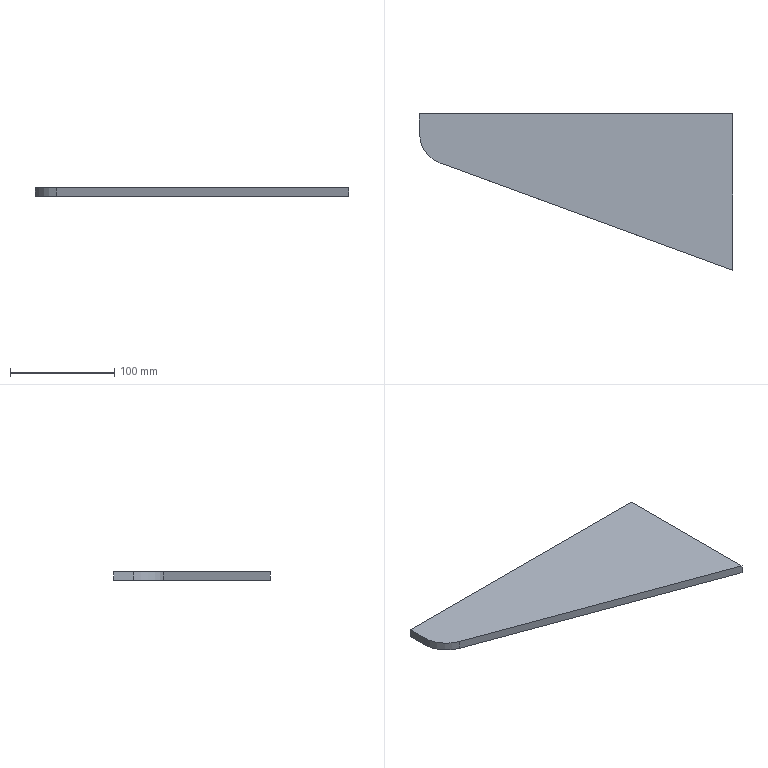Part | SolidWorks | features Extrusion 1 | 1 solid | 7 faces | box 300 x 150 x 8 mm | volume 227361 mm3 | plane 6 | cylinder 1 | commonest cylinder face diameters 60 x1
STEP:
#1=CARTESIAN_POINT('',(330.,-150.,0.));
#2=VERTEX_POINT('',#1);
#3=CARTESIAN_POINT('',(330.,0.,0.));
#4=VERTEX_POINT('',#3);
#5=CARTESIAN_POINT('',(330.,0.,0.));
#6=DIRECTION('',(0.,1.,0.));
#7=VECTOR('',#6,1000.);
#8=LINE('',#5,#7);
#9=EDGE_CURVE('',#2,#4,#8,.T.);
#10=ORIENTED_EDGE('',*,*,#9,.T.);
#11=CARTESIAN_POINT('',(330.,0.,8.));
#12=VERTEX_POINT('',#11);
#13=CARTESIAN_POINT('',(330.,0.,8.));
#14=DIRECTION('',(0.,0.,-1.));
#15=VECTOR('',#14,1000.);
#16=LINE('',#13,#15);
#17=EDGE_CURVE('',#12,#4,#16,.T.);
#18=ORIENTED_EDGE('',*,*,#17,.F.);
#19=CARTESIAN_POINT('',(330.,-150.,8.));
#20=VERTEX_POINT('',#19);
#21=CARTESIAN_POINT('',(330.,0.,8.));
#22=DIRECTION('',(0.,1.,0.));
#23=VECTOR('',#22,1000.);
#24=LINE('',#21,#23);
#25=EDGE_CURVE('',#20,#12,#24,.T.);
#26=ORIENTED_EDGE('',*,*,#25,.F.);
#27=CARTESIAN_POINT('',(330.,-150.,8.));
#28=DIRECTION('',(0.,0.,-1.));
#29=VECTOR('',#28,1000.);
#30=LINE('',#27,#29);
#31=EDGE_CURVE('',#20,#2,#30,.T.);
#32=ORIENTED_EDGE('',*,*,#31,.T.);
#33=EDGE_LOOP('',(#10,#18,#26,#32));
#34=FACE_OUTER_BOUND('',#33,.T.);
#35=CARTESIAN_POINT('',(330.,0.,8.));
#36=DIRECTION('',(-1.,0.,0.));
#37=DIRECTION('',(0.,0.,1.));
#38=AXIS2_PLACEMENT_3D('',#35,#36,#37);
#39=PLANE('',#38);
#40=ADVANCED_FACE('',(#34),#39,.F.);
#41=CARTESIAN_POINT('',(30.,0.,0.));
#42=VERTEX_POINT('',#41);
#43=CARTESIAN_POINT('',(330.,0.,0.));
#44=DIRECTION('',(-1.,0.,0.));
#45=VECTOR('',#44,1000.);
#46=LINE('',#43,#45);
#47=EDGE_CURVE('',#4,#42,#46,.T.);
#48=ORIENTED_EDGE('',*,*,#47,.T.);
#49=CARTESIAN_POINT('',(30.,0.,8.));
#50=VERTEX_POINT('',#49);
#51=CARTESIAN_POINT('',(30.,0.,8.));
#52=DIRECTION('',(0.,0.,-1.));
#53=VECTOR('',#52,1000.);
#54=LINE('',#51,#53);
#55=EDGE_CURVE('',#50,#42,#54,.T.);
#56=ORIENTED_EDGE('',*,*,#55,.F.);
#57=CARTESIAN_POINT('',(330.,0.,8.));
#58=DIRECTION('',(-1.,0.,0.));
#59=VECTOR('',#58,1000.);
#60=LINE('',#57,#59);
#61=EDGE_CURVE('',#12,#50,#60,.T.);
#62=ORIENTED_EDGE('',*,*,#61,.F.);
#63=ORIENTED_EDGE('',*,*,#17,.T.);
#64=EDGE_LOOP('',(#48,#56,#62,#63));
#65=FACE_OUTER_BOUND('',#64,.T.);
#66=CARTESIAN_POINT('',(330.,0.,8.));
#67=DIRECTION('',(0.,-1.,0.));
#68=DIRECTION('',(1.,0.,0.));
#69=AXIS2_PLACEMENT_3D('',#66,#67,#68);
#70=PLANE('',#69);
#71=ADVANCED_FACE('',(#65),#70,.F.);
#72=CARTESIAN_POINT('',(30.,-19.047,0.));
#73=VERTEX_POINT('',#72);
#74=CARTESIAN_POINT('',(30.,0.,0.));
#75=DIRECTION('',(0.,-1.,0.));
#76=VECTOR('',#75,1000.);
#77=LINE('',#74,#76);
#78=EDGE_CURVE('',#42,#73,#77,.T.);
#79=ORIENTED_EDGE('',*,*,#78,.T.);
#80=CARTESIAN_POINT('',(30.,-19.047,8.));
#81=VERTEX_POINT('',#80);
#82=CARTESIAN_POINT('',(30.,-19.047,8.));
#83=DIRECTION('',(0.,0.,-1.));
#84=VECTOR('',#83,1000.);
#85=LINE('',#82,#84);
#86=EDGE_CURVE('',#81,#73,#85,.T.);
#87=ORIENTED_EDGE('',*,*,#86,.F.);
#88=CARTESIAN_POINT('',(30.,0.,8.));
#89=DIRECTION('',(0.,-1.,0.));
#90=VECTOR('',#89,1000.);
#91=LINE('',#88,#90);
#92=EDGE_CURVE('',#50,#81,#91,.T.);
#93=ORIENTED_EDGE('',*,*,#92,.F.);
#94=ORIENTED_EDGE('',*,*,#55,.T.);
#95=EDGE_LOOP('',(#79,#87,#93,#94));
#96=FACE_OUTER_BOUND('',#95,.T.);
#97=CARTESIAN_POINT('',(30.,0.,8.));
#98=DIRECTION('',(1.,0.,0.));
#99=DIRECTION('',(0.,0.,-1.));
#100=AXIS2_PLACEMENT_3D('',#97,#98,#99);
#101=PLANE('',#100);
#102=ADVANCED_FACE('',(#96),#101,.F.);
#103=CARTESIAN_POINT('',(49.672,-47.213,0.));
#104=VERTEX_POINT('',#103);
#105=CARTESIAN_POINT('',(60.,-19.047,0.));
#106=DIRECTION('',(0.,0.,1.));
#107=DIRECTION('',(1.,0.,0.));
#108=AXIS2_PLACEMENT_3D('',#105,#106,#107);
#109=CIRCLE('',#108,30.);
#110=EDGE_CURVE('',#73,#104,#109,.T.);
#111=ORIENTED_EDGE('',*,*,#110,.T.);
#112=CARTESIAN_POINT('',(49.672,-47.213,8.));
#113=VERTEX_POINT('',#112);
#114=CARTESIAN_POINT('',(49.672,-47.213,8.));
#115=DIRECTION('',(0.,0.,-1.));
#116=VECTOR('',#115,1000.);
#117=LINE('',#114,#116);
#118=EDGE_CURVE('',#113,#104,#117,.T.);
#119=ORIENTED_EDGE('',*,*,#118,.F.);
#120=CARTESIAN_POINT('',(60.,-19.047,8.));
#121=DIRECTION('',(0.,0.,1.));
#122=DIRECTION('',(1.,0.,0.));
#123=AXIS2_PLACEMENT_3D('',#120,#121,#122);
#124=CIRCLE('',#123,30.);
#125=EDGE_CURVE('',#81,#113,#124,.T.);
#126=ORIENTED_EDGE('',*,*,#125,.F.);
#127=ORIENTED_EDGE('',*,*,#86,.T.);
#128=EDGE_LOOP('',(#111,#119,#126,#127));
#129=FACE_OUTER_BOUND('',#128,.T.);
#130=CARTESIAN_POINT('',(60.,-19.047,8.));
#131=DIRECTION('',(0.,0.,-1.));
#132=DIRECTION('',(-1.,0.,0.));
#133=AXIS2_PLACEMENT_3D('',#130,#131,#132);
#134=CYLINDRICAL_SURFACE('',#133,30.);
#135=ADVANCED_FACE('',(#129),#134,.T.);
#136=CARTESIAN_POINT('',(49.672,-47.213,0.));
#137=DIRECTION('',(0.9389,-0.3443,0.));
#138=VECTOR('',#137,1000.);
#139=LINE('',#136,#138);
#140=EDGE_CURVE('',#104,#2,#139,.T.);
#141=ORIENTED_EDGE('',*,*,#140,.T.);
#142=ORIENTED_EDGE('',*,*,#31,.F.);
#143=CARTESIAN_POINT('',(49.672,-47.213,8.));
#144=DIRECTION('',(0.9389,-0.3443,0.));
#145=VECTOR('',#144,1000.);
#146=LINE('',#143,#145);
#147=EDGE_CURVE('',#113,#20,#146,.T.);
#148=ORIENTED_EDGE('',*,*,#147,.F.);
#149=ORIENTED_EDGE('',*,*,#118,.T.);
#150=EDGE_LOOP('',(#141,#142,#148,#149));
#151=FACE_OUTER_BOUND('',#150,.T.);
#152=CARTESIAN_POINT('',(49.672,-47.213,8.));
#153=DIRECTION('',(0.3443,0.9389,0.));
#154=DIRECTION('',(-0.9389,0.3443,0.));
#155=AXIS2_PLACEMENT_3D('',#152,#153,#154);
#156=PLANE('',#155);
#157=ADVANCED_FACE('',(#151),#156,.F.);
#158=ORIENTED_EDGE('',*,*,#25,.T.);
#159=ORIENTED_EDGE('',*,*,#61,.T.);
#160=ORIENTED_EDGE('',*,*,#92,.T.);
#161=ORIENTED_EDGE('',*,*,#125,.T.);
#162=ORIENTED_EDGE('',*,*,#147,.T.);
#163=EDGE_LOOP('',(#158,#159,#160,#161,#162));
#164=FACE_OUTER_BOUND('',#163,.T.);
#165=CARTESIAN_POINT('',(60.,-19.047,8.));
#166=DIRECTION('',(0.,0.,1.));
#167=DIRECTION('',(1.,0.,0.));
#168=AXIS2_PLACEMENT_3D('',#165,#166,#167);
#169=PLANE('',#168);
#170=ADVANCED_FACE('',(#164),#169,.T.);
#171=ORIENTED_EDGE('',*,*,#9,.F.);
#172=ORIENTED_EDGE('',*,*,#140,.F.);
#173=ORIENTED_EDGE('',*,*,#110,.F.);
#174=ORIENTED_EDGE('',*,*,#78,.F.);
#175=ORIENTED_EDGE('',*,*,#47,.F.);
#176=EDGE_LOOP('',(#171,#172,#173,#174,#175));
#177=FACE_OUTER_BOUND('',#176,.T.);
#178=CARTESIAN_POINT('',(60.,-19.047,0.));
#179=DIRECTION('',(0.,0.,1.));
#180=DIRECTION('',(1.,0.,0.));
#181=AXIS2_PLACEMENT_3D('',#178,#179,#180);
#182=PLANE('',#181);
#183=ADVANCED_FACE('',(#177),#182,.F.);
#184=CLOSED_SHELL('',(#40,#71,#102,#135,#157,#170,#183));
#185=MANIFOLD_SOLID_BREP('',#184);
#186=CARTESIAN_POINT('',(0.,0.,0.));
#187=DIRECTION('',(0.,0.,1.));
#188=DIRECTION('',(1.,0.,0.));
#189=AXIS2_PLACEMENT_3D('',#186,#187,#188);
#190=(LENGTH_UNIT()NAMED_UNIT(*)SI_UNIT(.MILLI.,.METRE.));
#191=UNCERTAINTY_MEASURE_WITH_UNIT(LENGTH_MEASURE(0.00001),#190,'','');
#192=(NAMED_UNIT(*)PLANE_ANGLE_UNIT()SI_UNIT($,.RADIAN.));
#193=(NAMED_UNIT(*)SI_UNIT($,.STERADIAN.)SOLID_ANGLE_UNIT());
#194=(GEOMETRIC_REPRESENTATION_CONTEXT(3)GLOBAL_UNCERTAINTY_ASSIGNED_CONTEXT((#191))GLOBAL_UNIT_ASSIGNED_CONTEXT((#190,#192,#193))REPRESENTATION_CONTEXT('',''));
#195=ADVANCED_BREP_SHAPE_REPRESENTATION('',(#185,#189),#194);